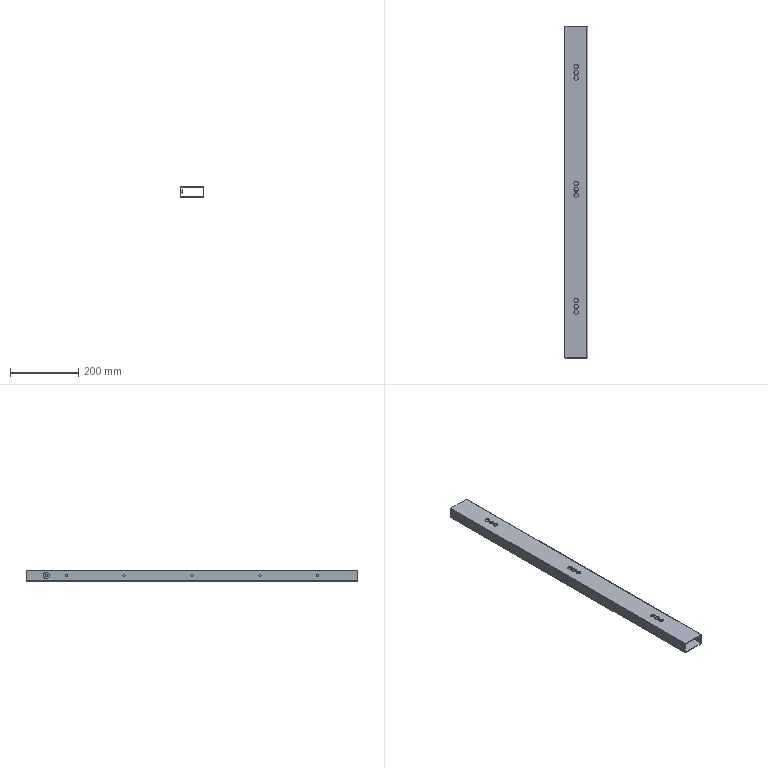Part | SolidWorks | features BaseBody 1 | 1 solid | 83 faces | box 70 x 976 x 33 mm | volume 377663 mm3 | cylinder 50 | plane 33 | commonest cylinder face diameters 6.5 x22 13 x18 6 x5 2 x3 18 x2